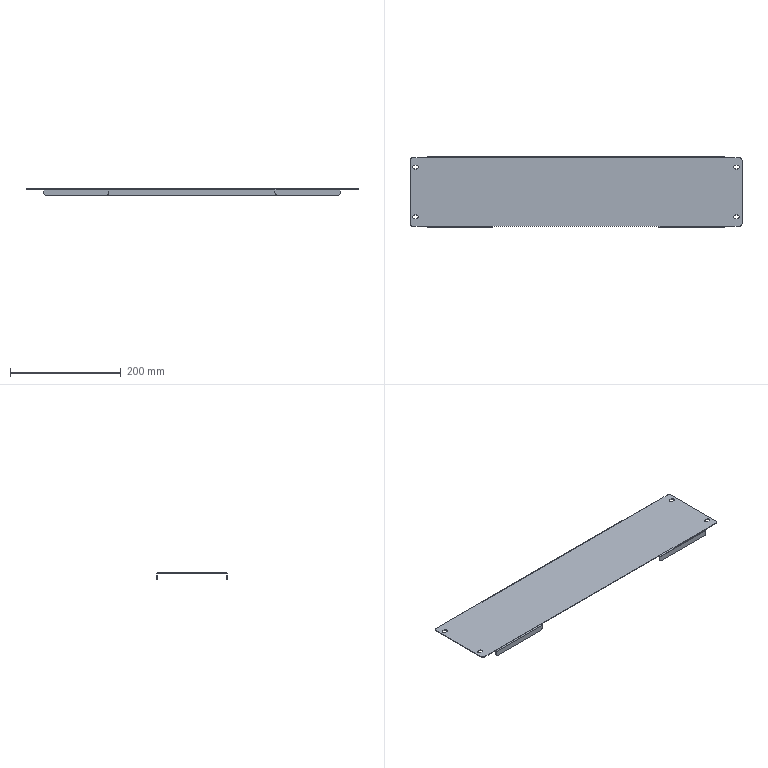Part | SolidWorks | features BaseBody 1 | 1 solid | 63 faces | box 600 x 128 x 12 mm | volume 83647 mm3 | plane 35 | cylinder 28 | commonest cylinder face diameters 7 x12 10 x10 2 x3 4 x3